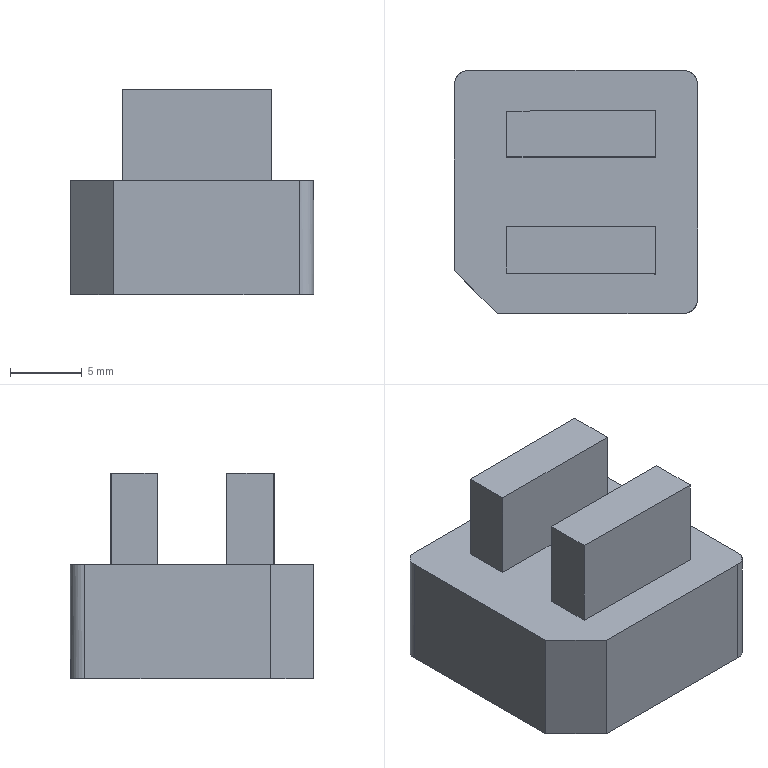CAM job | PowerMill | 3-axis milling, other | part box 17 x 17 x 14.396 mm
Tools:
number,name,type,diameter,tip_radius,length,cutting_length,overhang,flutes,holder,toolpaths_using
1,D10C,end_mill,10.0,0.0,60.0,,30.0,1,D42L35,2
10,D3_3,end_mill,3.0,0.0,30.0,,6.44,1,D42L35,2
1,D10C_1_1,end_mill,10.0,0.0,60.0,,14.84,1,D42L35,6
15,D3C_1_1,end_mill,3.0,0.0,30.0,,6.6,1,D42L35,1
3,D10_1_1,end_mill,10.0,0.0,60.0,,14.56,1,D42L35,8
10,D3_1_1,end_mill,3.0,0.0,30.0,,6.56,1,D42L35,2
13,Text_D4_1_1,taper_spherical,4.0,0.3,60.0,,6.64,1,D42L35,2
15,D3C_2_1,end_mill,3.0,0.0,30.0,,6.44,1,D42L35,1
Operations:
program,toolpath,strategy,tool,tool_number,tool_diameter,tip_radius,flutes,spindle_rpm,feed_cut,surface_speed_m_min_computed,feed_per_tooth_computed,tolerance,thickness,stepover,stepdown,cut_length,cut_time_min,total_time_min,workplane
001-D-10-F,精公开粗01-扫面平行-D10C,raster_area_clear,D10C_1_1,1,10.0,0.0,1.0,8000.0,10000.0,251.33,1.25,0.03,0.28,6.0,1.0,135.36,0.013,0.0178,
001-D-10-F,精公开粗01-外形偏置-D10C,offset_area_clear,D10C_1_1,1,10.0,0.0,1.0,8000.0,10000.0,251.33,1.25,0.03,0.28,6.0,1.0,2979.625,0.298,0.3395,
001-D-10-F,精公开粗01-基准台等高-D10C,constantz,D10C_1_1,1,10.0,0.0,1.0,8000.0,10000.0,251.33,1.25,0.03,0.07,5.0,0.4,2129.073,0.213,0.2212,
001-D-10-F,精公再粗02-外形偏置-D3C,offset_area_clear,D3C_1_1,15,3.0,0.0,1.0,18000.0,5000.0,169.65,0.2778,0.03,0.0,2.0,1.0,3510.67,0.702,0.958,
001-D-10-F,精公基准台01-平坦面平行-D10,raster_area_clear,D10_1_1,3,10.0,0.0,1.0,8500.0,600.0,267.04,0.0706,0.005,0.38,5.0,1.0,98.646,0.164,0.1806,
001-D-10-F,精公基准台01-基准面偏置-D10,offset_area_clear,D10_1_1,3,10.0,0.0,1.0,8500.0,600.0,267.04,0.0706,0.005,0.38,5.0,1.0,84.101,0.14,0.1575,
001-D-10-F,精公基准台01-外形侧光-D10,profile_area_clear,D10_1_1,3,10.0,0.0,1.0,8500.0,600.0,267.04,0.0706,0.005,-0.07,0.08,1.0,150.332,0.251,0.2698,
001-D-10-F,精公基准台01-基准台侧光-D10,profile_area_clear,D10_1_1,3,10.0,0.0,1.0,8500.0,600.0,267.04,0.0706,0.005,0.0,0.08,1.0,193.234,0.322,0.3848,
001-D-10-F,精公精光01-等高-D3,constantz,D3_1_1,10,3.0,0.0,1.0,18000.0,2000.0,169.65,0.1111,0.005,-0.075,5.0,0.03,15377.451,7.689,7.698,
001-D-10-F,精公精光01-平坦面平行-D3,raster_area_clear,D3_1_1,10,3.0,0.0,1.0,18000.0,600.0,169.65,0.0333,0.005,0.375,1.5,1.0,122.896,0.205,0.2213,
001-D-10-F,精公刻字01-刻字-Text_D4,pattern,Text_D4_1_1,13,4.0,0.3,1.0,15000.0,1000.0,188.5,0.0667,0.005,0.0,5.0,1.0,16.465,0.017,0.0318,
001-D-10-R,粗公开粗01-扫面平行-D10C,raster_area_clear,D10C_1_1,1,10.0,0.0,1.0,8000.0,10000.0,251.33,1.25,0.03,0.15,6.0,1.0,267.6,0.027,0.0329,
001-D-10-R,粗公开粗01-外形偏置-D10C,offset_area_clear,D10C_1_1,1,10.0,0.0,1.0,8000.0,10000.0,251.33,1.25,0.03,0.15,6.0,1.0,2950.23,0.295,0.3366,
001-D-10-R,粗公开粗01-基准台等高-D10C,constantz,D10C_1_1,1,10.0,0.0,1.0,8000.0,10000.0,251.33,1.25,0.03,0.07,5.0,0.4,2129.073,0.213,0.2212,
001-D-10-R,粗公再粗02-外形偏置-D3C,offset_area_clear,D3C_2_1,15,3.0,0.0,1.0,18000.0,5000.0,169.65,0.2778,0.03,-0.13,2.0,1.0,3202.716,0.64,0.8797,
001-D-10-R,粗公基准台01-平坦面平行-D10,raster_area_clear,D10_1_1,3,10.0,0.0,1.0,8500.0,600.0,267.04,0.0706,0.01,0.25,5.0,1.0,97.49,0.163,0.1787,
001-D-10-R,粗公基准台01-基准面偏置-D10,offset_area_clear,D10_1_1,3,10.0,0.0,1.0,8500.0,600.0,267.04,0.0706,0.01,0.25,5.0,1.0,83.29,0.139,0.1561,
001-D-10-R,粗公基准台01-外形侧光-D10,profile_area_clear,D10_1_1,3,10.0,0.0,1.0,8500.0,600.0,267.04,0.0706,0.01,-0.2,0.08,1.0,148.742,0.248,0.2672,
001-D-10-R,粗公基准台01-基准台侧光-D10,profile_area_clear,D10_1_1,3,10.0,0.0,1.0,8500.0,600.0,267.04,0.0706,0.01,0.0,0.08,1.0,193.218,0.322,0.3848,
001-D-10-R,粗公精光01-等高-D3,constantz,D3_3,10,3.0,0.0,1.0,18000.0,2000.0,169.65,0.1111,0.01,-0.205,5.0,0.036,12265.46,6.133,6.142,
001-D-10-R,粗公精光01-平坦面平行-D3,raster_area_clear,D3_3,10,3.0,0.0,1.0,18000.0,600.0,169.65,0.0333,0.01,0.245,1.5,1.0,120.627,0.201,0.2176,
001-D-10-R,粗公刻字01-刻字-Text_D4,pattern,Text_D4_1_1,13,4.0,0.3,1.0,15000.0,1000.0,188.5,0.0667,0.01,0.0,5.0,1.0,15.92,0.016,0.0304,
,精公开粗01-外形偏置-D10C_Reference,offset_area_clear,D10C,1,10.0,0.0,1.0,8000.0,10000.0,251.33,1.25,0.03,0.28,6.0,1.0,7821.009,0.782,0.8867,
,粗公开粗01-外形偏置-D10C_Reference,offset_area_clear,D10C,1,10.0,0.0,1.0,8000.0,10000.0,251.33,1.25,0.03,0.15,6.0,1.0,7743.909,0.774,0.8794,